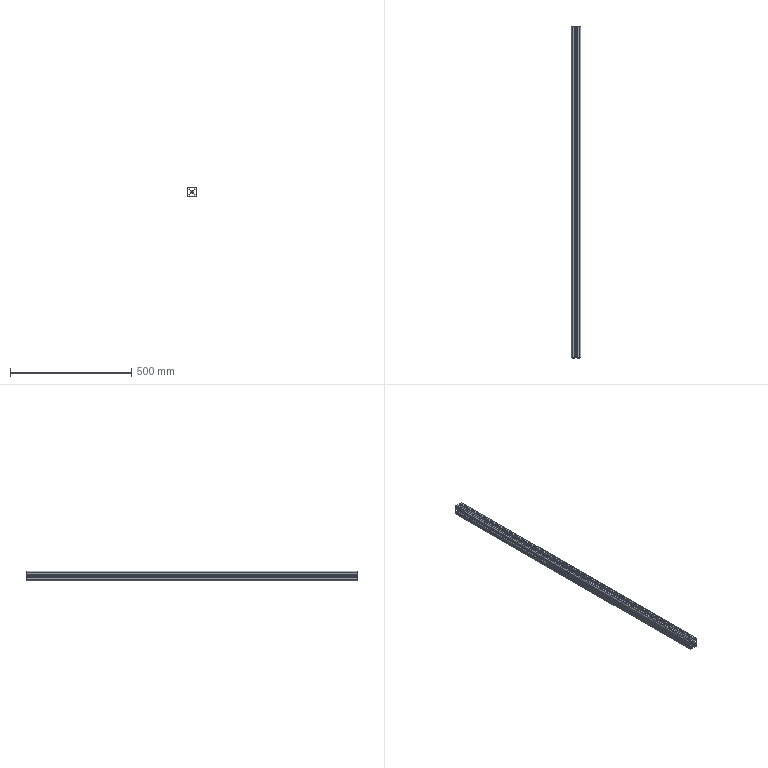Part | 1 solid | 104 faces | box 40 x 1370 x 40 mm | volume 789867 mm3 | plane 94 | cylinder 10 | commonest cylinder face diameters 5 x4 9 x4 6.8 x2